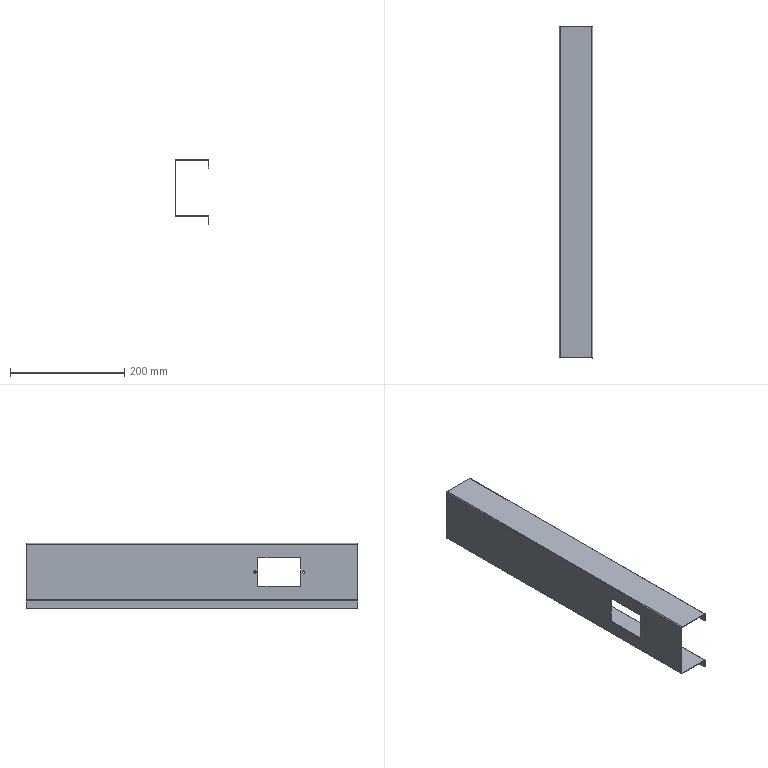Part | SolidWorks | features EdgeFlange 2, FlatPattern 1, ICE 1, SMBaseFlange 1, SheetMetal 1 | 1 solid | 46 faces | box 58.8 x 580 x 113.8 mm | volume 163204 mm3 | plane 34 | cylinder 12 | commonest cylinder face diameters 0.9 x4 3.3 x4 4 x4
STEP:
#1=CARTESIAN_POINT('',(0.,-110.,2.));
#2=VERTEX_POINT('',#1);
#3=CARTESIAN_POINT('',(0.,-110.,-2.));
#4=VERTEX_POINT('',#3);
#5=CARTESIAN_POINT('',(0.,-110.,0.));
#6=DIRECTION('',(1.,0.,0.));
#7=DIRECTION('',(0.,0.,-1.));
#8=AXIS2_PLACEMENT_3D('',#5,#6,#7);
#9=CIRCLE('',#8,2.);
#10=EDGE_CURVE('',#2,#4,#9,.T.);
#11=ORIENTED_EDGE('',*,*,#10,.F.);
#12=CARTESIAN_POINT('',(1.2,-110.,2.));
#13=VERTEX_POINT('',#12);
#14=CARTESIAN_POINT('',(-8.8,-110.,2.));
#15=DIRECTION('',(1.,0.,0.));
#16=VECTOR('',#15,1000.);
#17=LINE('',#14,#16);
#18=EDGE_CURVE('',#2,#13,#17,.T.);
#19=ORIENTED_EDGE('',*,*,#18,.T.);
#20=CARTESIAN_POINT('',(1.2,-110.,-2.));
#21=VERTEX_POINT('',#20);
#22=CARTESIAN_POINT('',(1.2,-110.,0.));
#23=DIRECTION('',(1.,0.,0.));
#24=DIRECTION('',(0.,0.,1.));
#25=AXIS2_PLACEMENT_3D('',#22,#23,#24);
#26=CIRCLE('',#25,2.);
#27=EDGE_CURVE('',#13,#21,#26,.T.);
#28=ORIENTED_EDGE('',*,*,#27,.T.);
#29=CARTESIAN_POINT('',(-8.8,-110.,-2.));
#30=DIRECTION('',(1.,0.,0.));
#31=VECTOR('',#30,1000.);
#32=LINE('',#29,#31);
#33=EDGE_CURVE('',#4,#21,#32,.T.);
#34=ORIENTED_EDGE('',*,*,#33,.F.);
#35=EDGE_LOOP('',(#11,#19,#28,#34));
#36=FACE_OUTER_BOUND('',#35,.T.);
#37=CARTESIAN_POINT('',(-8.8,-110.,0.));
#38=DIRECTION('',(1.,0.,0.));
#39=DIRECTION('',(0.,0.,-1.));
#40=AXIS2_PLACEMENT_3D('',#37,#38,#39);
#41=CYLINDRICAL_SURFACE('',#40,2.);
#42=ADVANCED_FACE('',(#36),#41,.F.);
#43=CARTESIAN_POINT('',(0.,-195.,2.));
#44=VERTEX_POINT('',#43);
#45=CARTESIAN_POINT('',(0.,-195.,-2.));
#46=VERTEX_POINT('',#45);
#47=CARTESIAN_POINT('',(0.,-195.,0.));
#48=DIRECTION('',(1.,0.,0.));
#49=DIRECTION('',(0.,0.,-1.));
#50=AXIS2_PLACEMENT_3D('',#47,#48,#49);
#51=CIRCLE('',#50,2.);
#52=EDGE_CURVE('',#44,#46,#51,.T.);
#53=ORIENTED_EDGE('',*,*,#52,.F.);
#54=CARTESIAN_POINT('',(1.2,-195.,2.));
#55=VERTEX_POINT('',#54);
#56=CARTESIAN_POINT('',(-8.8,-195.,2.));
#57=DIRECTION('',(1.,0.,0.));
#58=VECTOR('',#57,1000.);
#59=LINE('',#56,#58);
#60=EDGE_CURVE('',#44,#55,#59,.T.);
#61=ORIENTED_EDGE('',*,*,#60,.T.);
#62=CARTESIAN_POINT('',(1.2,-195.,-2.));
#63=VERTEX_POINT('',#62);
#64=CARTESIAN_POINT('',(1.2,-195.,0.));
#65=DIRECTION('',(1.,0.,0.));
#66=DIRECTION('',(0.,0.,-1.));
#67=AXIS2_PLACEMENT_3D('',#64,#65,#66);
#68=CIRCLE('',#67,2.);
#69=EDGE_CURVE('',#55,#63,#68,.T.);
#70=ORIENTED_EDGE('',*,*,#69,.T.);
#71=CARTESIAN_POINT('',(-8.8,-195.,-2.));
#72=DIRECTION('',(1.,0.,0.));
#73=VECTOR('',#72,1000.);
#74=LINE('',#71,#73);
#75=EDGE_CURVE('',#46,#63,#74,.T.);
#76=ORIENTED_EDGE('',*,*,#75,.F.);
#77=EDGE_LOOP('',(#53,#61,#70,#76));
#78=FACE_OUTER_BOUND('',#77,.T.);
#79=CARTESIAN_POINT('',(-8.8,-195.,0.));
#80=DIRECTION('',(1.,0.,0.));
#81=DIRECTION('',(0.,0.,-1.));
#82=AXIS2_PLACEMENT_3D('',#79,#80,#81);
#83=CYLINDRICAL_SURFACE('',#82,2.);
#84=ADVANCED_FACE('',(#78),#83,.F.);
#85=CARTESIAN_POINT('',(57.15,290.,-50.));
#86=VERTEX_POINT('',#85);
#87=CARTESIAN_POINT('',(57.15,290.,-48.8));
#88=VERTEX_POINT('',#87);
#89=CARTESIAN_POINT('',(57.15,290.,-50.));
#90=DIRECTION('',(0.,0.,1.));
#91=VECTOR('',#90,1000.);
#92=LINE('',#89,#91);
#93=EDGE_CURVE('',#86,#88,#92,.T.);
#94=ORIENTED_EDGE('',*,*,#93,.F.);
#95=CARTESIAN_POINT('',(1.65,290.,-50.));
#96=VERTEX_POINT('',#95);
#97=CARTESIAN_POINT('',(1.2,290.,-50.));
#98=DIRECTION('',(1.,0.,0.));
#99=VECTOR('',#98,1000.);
#100=LINE('',#97,#99);
#101=EDGE_CURVE('',#96,#86,#100,.T.);
#102=ORIENTED_EDGE('',*,*,#101,.F.);
#103=CARTESIAN_POINT('',(1.65,290.,-48.8));
#104=VERTEX_POINT('',#103);
#105=CARTESIAN_POINT('',(1.65,290.,-48.8));
#106=DIRECTION('',(0.,0.,-1.));
#107=VECTOR('',#106,1000.);
#108=LINE('',#105,#107);
#109=EDGE_CURVE('',#104,#96,#108,.T.);
#110=ORIENTED_EDGE('',*,*,#109,.F.);
#111=CARTESIAN_POINT('',(1.2,290.,-48.8));
#112=DIRECTION('',(1.,0.,0.));
#113=VECTOR('',#112,1000.);
#114=LINE('',#111,#113);
#115=EDGE_CURVE('',#104,#88,#114,.T.);
#116=ORIENTED_EDGE('',*,*,#115,.T.);
#117=EDGE_LOOP('',(#94,#102,#110,#116));
#118=FACE_OUTER_BOUND('',#117,.T.);
#119=CARTESIAN_POINT('',(1.2,290.,-50.));
#120=DIRECTION('',(0.,-1.,0.));
#121=DIRECTION('',(0.,0.,-1.));
#122=AXIS2_PLACEMENT_3D('',#119,#120,#121);
#123=PLANE('',#122);
#124=ADVANCED_FACE('',(#118),#123,.F.);
#125=CARTESIAN_POINT('',(57.15,-290.,-50.));
#126=VERTEX_POINT('',#125);
#127=CARTESIAN_POINT('',(57.15,-290.,-48.8));
#128=VERTEX_POINT('',#127);
#129=CARTESIAN_POINT('',(57.15,-290.,-50.));
#130=DIRECTION('',(0.,0.,1.));
#131=VECTOR('',#130,1000.);
#132=LINE('',#129,#131);
#133=EDGE_CURVE('',#126,#128,#132,.T.);
#134=ORIENTED_EDGE('',*,*,#133,.T.);
#135=CARTESIAN_POINT('',(1.65,-290.,-48.8));
#136=VERTEX_POINT('',#135);
#137=CARTESIAN_POINT('',(58.8,-290.,-48.8));
#138=DIRECTION('',(-1.,0.,0.));
#139=VECTOR('',#138,1000.);
#140=LINE('',#137,#139);
#141=EDGE_CURVE('',#128,#136,#140,.T.);
#142=ORIENTED_EDGE('',*,*,#141,.T.);
#143=CARTESIAN_POINT('',(1.65,-290.,-50.));
#144=VERTEX_POINT('',#143);
#145=CARTESIAN_POINT('',(1.65,-290.,-50.));
#146=DIRECTION('',(0.,0.,-1.));
#147=VECTOR('',#146,1000.);
#148=LINE('',#145,#147);
#149=EDGE_CURVE('',#136,#144,#148,.T.);
#150=ORIENTED_EDGE('',*,*,#149,.T.);
#151=CARTESIAN_POINT('',(1.2,-290.,-50.));
#152=DIRECTION('',(-1.,0.,0.));
#153=VECTOR('',#152,1000.);
#154=LINE('',#151,#153);
#155=EDGE_CURVE('',#126,#144,#154,.T.);
#156=ORIENTED_EDGE('',*,*,#155,.F.);
#157=EDGE_LOOP('',(#134,#142,#150,#156));
#158=FACE_OUTER_BOUND('',#157,.T.);
#159=CARTESIAN_POINT('',(58.8,-290.,-50.));
#160=DIRECTION('',(0.,1.,0.));
#161=DIRECTION('',(0.,0.,1.));
#162=AXIS2_PLACEMENT_3D('',#159,#160,#161);
#163=PLANE('',#162);
#164=ADVANCED_FACE('',(#158),#163,.F.);
#165=ORIENTED_EDGE('',*,*,#101,.T.);
#166=CARTESIAN_POINT('',(57.15,-290.,-50.));
#167=DIRECTION('',(0.,1.,0.));
#168=VECTOR('',#167,1000.);
#169=LINE('',#166,#168);
#170=EDGE_CURVE('',#126,#86,#169,.T.);
#171=ORIENTED_EDGE('',*,*,#170,.F.);
#172=ORIENTED_EDGE('',*,*,#155,.T.);
#173=CARTESIAN_POINT('',(1.65,290.,-50.));
#174=DIRECTION('',(0.,1.,0.));
#175=VECTOR('',#174,1000.);
#176=LINE('',#173,#175);
#177=EDGE_CURVE('',#144,#96,#176,.T.);
#178=ORIENTED_EDGE('',*,*,#177,.T.);
#179=EDGE_LOOP('',(#165,#171,#172,#178));
#180=FACE_OUTER_BOUND('',#179,.T.);
#181=CARTESIAN_POINT('',(1.2,290.,-50.));
#182=DIRECTION('',(0.,0.,-1.));
#183=DIRECTION('',(-1.,0.,0.));
#184=AXIS2_PLACEMENT_3D('',#181,#182,#183);
#185=PLANE('',#184);
#186=ADVANCED_FACE('',(#180),#185,.T.);
#187=CARTESIAN_POINT('',(57.15,-290.,-48.8));
#188=DIRECTION('',(0.,1.,0.));
#189=VECTOR('',#188,1000.);
#190=LINE('',#187,#189);
#191=EDGE_CURVE('',#128,#88,#190,.T.);
#192=ORIENTED_EDGE('',*,*,#191,.T.);
#193=ORIENTED_EDGE('',*,*,#115,.F.);
#194=CARTESIAN_POINT('',(1.65,-290.,-48.8));
#195=DIRECTION('',(0.,1.,0.));
#196=VECTOR('',#195,1000.);
#197=LINE('',#194,#196);
#198=EDGE_CURVE('',#136,#104,#197,.T.);
#199=ORIENTED_EDGE('',*,*,#198,.F.);
#200=ORIENTED_EDGE('',*,*,#141,.F.);
#201=EDGE_LOOP('',(#192,#193,#199,#200));
#202=FACE_OUTER_BOUND('',#201,.T.);
#203=CARTESIAN_POINT('',(1.2,290.,-48.8));
#204=DIRECTION('',(0.,0.,-1.));
#205=DIRECTION('',(-1.,0.,0.));
#206=AXIS2_PLACEMENT_3D('',#203,#204,#205);
#207=PLANE('',#206);
#208=ADVANCED_FACE('',(#202),#207,.F.);
#209=CARTESIAN_POINT('',(57.15,-290.,48.8));
#210=VERTEX_POINT('',#209);
#211=CARTESIAN_POINT('',(57.15,-290.,50.));
#212=VERTEX_POINT('',#211);
#213=CARTESIAN_POINT('',(57.15,-290.,48.8));
#214=DIRECTION('',(0.,0.,1.));
#215=VECTOR('',#214,1000.);
#216=LINE('',#213,#215);
#217=EDGE_CURVE('',#210,#212,#216,.T.);
#218=ORIENTED_EDGE('',*,*,#217,.T.);
#219=CARTESIAN_POINT('',(1.65,-290.,50.));
#220=VERTEX_POINT('',#219);
#221=CARTESIAN_POINT('',(1.2,-290.,50.));
#222=DIRECTION('',(1.,0.,0.));
#223=VECTOR('',#222,1000.);
#224=LINE('',#221,#223);
#225=EDGE_CURVE('',#220,#212,#224,.T.);
#226=ORIENTED_EDGE('',*,*,#225,.F.);
#227=CARTESIAN_POINT('',(1.65,-290.,48.8));
#228=VERTEX_POINT('',#227);
#229=CARTESIAN_POINT('',(1.65,-290.,48.8));
#230=DIRECTION('',(0.,0.,1.));
#231=VECTOR('',#230,1000.);
#232=LINE('',#229,#231);
#233=EDGE_CURVE('',#228,#220,#232,.T.);
#234=ORIENTED_EDGE('',*,*,#233,.F.);
#235=CARTESIAN_POINT('',(58.8,-290.,48.8));
#236=DIRECTION('',(1.,0.,0.));
#237=VECTOR('',#236,1000.);
#238=LINE('',#235,#237);
#239=EDGE_CURVE('',#228,#210,#238,.T.);
#240=ORIENTED_EDGE('',*,*,#239,.T.);
#241=EDGE_LOOP('',(#218,#226,#234,#240));
#242=FACE_OUTER_BOUND('',#241,.T.);
#243=CARTESIAN_POINT('',(58.8,-290.,50.));
#244=DIRECTION('',(0.,1.,0.));
#245=DIRECTION('',(0.,0.,1.));
#246=AXIS2_PLACEMENT_3D('',#243,#244,#245);
#247=PLANE('',#246);
#248=ADVANCED_FACE('',(#242),#247,.F.);
#249=CARTESIAN_POINT('',(57.15,290.,48.8));
#250=VERTEX_POINT('',#249);
#251=CARTESIAN_POINT('',(57.15,290.,50.));
#252=VERTEX_POINT('',#251);
#253=CARTESIAN_POINT('',(57.15,290.,48.8));
#254=DIRECTION('',(0.,0.,1.));
#255=VECTOR('',#254,1000.);
#256=LINE('',#253,#255);
#257=EDGE_CURVE('',#250,#252,#256,.T.);
#258=ORIENTED_EDGE('',*,*,#257,.F.);
#259=CARTESIAN_POINT('',(1.65,290.,48.8));
#260=VERTEX_POINT('',#259);
#261=CARTESIAN_POINT('',(1.2,290.,48.8));
#262=DIRECTION('',(-1.,0.,0.));
#263=VECTOR('',#262,1000.);
#264=LINE('',#261,#263);
#265=EDGE_CURVE('',#250,#260,#264,.T.);
#266=ORIENTED_EDGE('',*,*,#265,.T.);
#267=CARTESIAN_POINT('',(1.65,290.,50.));
#268=VERTEX_POINT('',#267);
#269=CARTESIAN_POINT('',(1.65,290.,50.));
#270=DIRECTION('',(0.,0.,1.));
#271=VECTOR('',#270,1000.);
#272=LINE('',#269,#271);
#273=EDGE_CURVE('',#260,#268,#272,.T.);
#274=ORIENTED_EDGE('',*,*,#273,.T.);
#275=CARTESIAN_POINT('',(1.2,290.,50.));
#276=DIRECTION('',(-1.,0.,0.));
#277=VECTOR('',#276,1000.);
#278=LINE('',#275,#277);
#279=EDGE_CURVE('',#252,#268,#278,.T.);
#280=ORIENTED_EDGE('',*,*,#279,.F.);
#281=EDGE_LOOP('',(#258,#266,#274,#280));
#282=FACE_OUTER_BOUND('',#281,.T.);
#283=CARTESIAN_POINT('',(1.2,290.,50.));
#284=DIRECTION('',(0.,-1.,0.));
#285=DIRECTION('',(0.,0.,-1.));
#286=AXIS2_PLACEMENT_3D('',#283,#284,#285);
#287=PLANE('',#286);
#288=ADVANCED_FACE('',(#282),#287,.F.);
#289=CARTESIAN_POINT('',(57.15,-290.,50.));
#290=DIRECTION('',(0.,1.,0.));
#291=VECTOR('',#290,1000.);
#292=LINE('',#289,#291);
#293=EDGE_CURVE('',#212,#252,#292,.T.);
#294=ORIENTED_EDGE('',*,*,#293,.T.);
#295=ORIENTED_EDGE('',*,*,#279,.T.);
#296=CARTESIAN_POINT('',(1.65,290.,50.));
#297=DIRECTION('',(0.,1.,0.));
#298=VECTOR('',#297,1000.);
#299=LINE('',#296,#298);
#300=EDGE_CURVE('',#220,#268,#299,.T.);
#301=ORIENTED_EDGE('',*,*,#300,.F.);
#302=ORIENTED_EDGE('',*,*,#225,.T.);
#303=EDGE_LOOP('',(#294,#295,#301,#302));
#304=FACE_OUTER_BOUND('',#303,.T.);
#305=CARTESIAN_POINT('',(1.2,-290.,50.));
#306=DIRECTION('',(0.,0.,-1.));
#307=DIRECTION('',(-1.,0.,0.));
#308=AXIS2_PLACEMENT_3D('',#305,#306,#307);
#309=PLANE('',#308);
#310=ADVANCED_FACE('',(#304),#309,.F.);
#311=ORIENTED_EDGE('',*,*,#265,.F.);
#312=CARTESIAN_POINT('',(57.15,-290.,48.8));
#313=DIRECTION('',(0.,1.,0.));
#314=VECTOR('',#313,1000.);
#315=LINE('',#312,#314);
#316=EDGE_CURVE('',#210,#250,#315,.T.);
#317=ORIENTED_EDGE('',*,*,#316,.F.);
#318=ORIENTED_EDGE('',*,*,#239,.F.);
#319=CARTESIAN_POINT('',(1.65,290.,48.8));
#320=DIRECTION('',(0.,-1.,0.));
#321=VECTOR('',#320,1000.);
#322=LINE('',#319,#321);
#323=EDGE_CURVE('',#260,#228,#322,.T.);
#324=ORIENTED_EDGE('',*,*,#323,.F.);
#325=EDGE_LOOP('',(#311,#317,#318,#324));
#326=FACE_OUTER_BOUND('',#325,.T.);
#327=CARTESIAN_POINT('',(1.2,-290.,48.8));
#328=DIRECTION('',(0.,0.,-1.));
#329=DIRECTION('',(-1.,0.,0.));
#330=AXIS2_PLACEMENT_3D('',#327,#328,#329);
#331=PLANE('',#330);
#332=ADVANCED_FACE('',(#326),#331,.T.);
#333=CARTESIAN_POINT('',(1.2,-290.,-48.35));
#334=VERTEX_POINT('',#333);
#335=CARTESIAN_POINT('',(0.,-290.,-48.35));
#336=VERTEX_POINT('',#335);
#337=CARTESIAN_POINT('',(1.2,-290.,-48.35));
#338=DIRECTION('',(-1.,0.,0.));
#339=VECTOR('',#338,1000.);
#340=LINE('',#337,#339);
#341=EDGE_CURVE('',#334,#336,#340,.T.);
#342=ORIENTED_EDGE('',*,*,#341,.F.);
#343=CARTESIAN_POINT('',(1.2,-290.,48.35));
#344=VERTEX_POINT('',#343);
#345=CARTESIAN_POINT('',(1.2,-290.,50.));
#346=DIRECTION('',(0.,0.,-1.));
#347=VECTOR('',#346,1000.);
#348=LINE('',#345,#347);
#349=EDGE_CURVE('',#344,#334,#348,.T.);
#350=ORIENTED_EDGE('',*,*,#349,.F.);
#351=CARTESIAN_POINT('',(0.,-290.,48.35));
#352=VERTEX_POINT('',#351);
#353=CARTESIAN_POINT('',(1.2,-290.,48.35));
#354=DIRECTION('',(-1.,0.,0.));
#355=VECTOR('',#354,1000.);
#356=LINE('',#353,#355);
#357=EDGE_CURVE('',#344,#352,#356,.T.);
#358=ORIENTED_EDGE('',*,*,#357,.T.);
#359=CARTESIAN_POINT('',(0.,-290.,50.));
#360=DIRECTION('',(0.,0.,-1.));
#361=VECTOR('',#360,1000.);
#362=LINE('',#359,#361);
#363=EDGE_CURVE('',#352,#336,#362,.T.);
#364=ORIENTED_EDGE('',*,*,#363,.T.);
#365=EDGE_LOOP('',(#342,#350,#358,#364));
#366=FACE_OUTER_BOUND('',#365,.T.);
#367=CARTESIAN_POINT('',(1.2,-290.,50.));
#368=DIRECTION('',(0.,1.,0.));
#369=DIRECTION('',(0.,0.,1.));
#370=AXIS2_PLACEMENT_3D('',#367,#368,#369);
#371=PLANE('',#370);
#372=ADVANCED_FACE('',(#366),#371,.F.);
#373=CARTESIAN_POINT('',(1.2,290.,-48.35));
#374=VERTEX_POINT('',#373);
#375=CARTESIAN_POINT('',(0.,290.,-48.35));
#376=VERTEX_POINT('',#375);
#377=CARTESIAN_POINT('',(1.2,290.,-48.35));
#378=DIRECTION('',(-1.,0.,0.));
#379=VECTOR('',#378,1000.);
#380=LINE('',#377,#379);
#381=EDGE_CURVE('',#374,#376,#380,.T.);
#382=ORIENTED_EDGE('',*,*,#381,.T.);
#383=CARTESIAN_POINT('',(0.,290.,48.35));
#384=VERTEX_POINT('',#383);
#385=CARTESIAN_POINT('',(0.,290.,50.));
#386=DIRECTION('',(0.,0.,1.));
#387=VECTOR('',#386,1000.);
#388=LINE('',#385,#387);
#389=EDGE_CURVE('',#376,#384,#388,.T.);
#390=ORIENTED_EDGE('',*,*,#389,.T.);
#391=CARTESIAN_POINT('',(1.2,290.,48.35));
#392=VERTEX_POINT('',#391);
#393=CARTESIAN_POINT('',(1.2,290.,48.35));
#394=DIRECTION('',(-1.,0.,0.));
#395=VECTOR('',#394,1000.);
#396=LINE('',#393,#395);
#397=EDGE_CURVE('',#392,#384,#396,.T.);
#398=ORIENTED_EDGE('',*,*,#397,.F.);
#399=CARTESIAN_POINT('',(1.2,290.,50.));
#400=DIRECTION('',(0.,0.,1.));
#401=VECTOR('',#400,1000.);
#402=LINE('',#399,#401);
#403=EDGE_CURVE('',#374,#392,#402,.T.);
#404=ORIENTED_EDGE('',*,*,#403,.F.);
#405=EDGE_LOOP('',(#382,#390,#398,#404));
#406=FACE_OUTER_BOUND('',#405,.T.);
#407=CARTESIAN_POINT('',(1.2,290.,50.));
#408=DIRECTION('',(0.,-1.,0.));
#409=DIRECTION('',(0.,0.,-1.));
#410=AXIS2_PLACEMENT_3D('',#407,#408,#409);
#411=PLANE('',#410);
#412=ADVANCED_FACE('',(#406),#411,.F.);
#413=CARTESIAN_POINT('',(1.2,-110.,0.));
#414=DIRECTION('',(1.,0.,0.));
#415=DIRECTION('',(0.,0.,1.));
#416=AXIS2_PLACEMENT_3D('',#413,#414,#415);
#417=CIRCLE('',#416,2.);
#418=EDGE_CURVE('',#21,#13,#417,.T.);
#419=ORIENTED_EDGE('',*,*,#418,.F.);
#420=ORIENTED_EDGE('',*,*,#27,.F.);
#421=EDGE_LOOP('',(#419,#420));
#422=FACE_BOUND('',#421,.T.);
#423=CARTESIAN_POINT('',(1.2,-195.,0.));
#424=DIRECTION('',(1.,0.,0.));
#425=DIRECTION('',(0.,0.,-1.));
#426=AXIS2_PLACEMENT_3D('',#423,#424,#425);
#427=CIRCLE('',#426,2.);
#428=EDGE_CURVE('',#63,#55,#427,.T.);
#429=ORIENTED_EDGE('',*,*,#428,.F.);
#430=ORIENTED_EDGE('',*,*,#69,.F.);
#431=EDGE_LOOP('',(#429,#430));
#432=FACE_BOUND('',#431,.T.);
#433=CARTESIAN_POINT('',(1.2,-115.,25.));
#434=VERTEX_POINT('',#433);
#435=CARTESIAN_POINT('',(1.2,-190.,25.));
#436=VERTEX_POINT('',#435);
#437=CARTESIAN_POINT('',(1.2,-115.,25.));
#438=DIRECTION('',(0.,-1.,0.));
#439=VECTOR('',#438,1000.);
#440=LINE('',#437,#439);
#441=EDGE_CURVE('',#434,#436,#440,.T.);
#442=ORIENTED_EDGE('',*,*,#441,.F.);
#443=CARTESIAN_POINT('',(1.2,-115.,-25.));
#444=VERTEX_POINT('',#443);
#445=CARTESIAN_POINT('',(1.2,-115.,25.));
#446=DIRECTION('',(0.,0.,1.));
#447=VECTOR('',#446,1000.);
#448=LINE('',#445,#447);
#449=EDGE_CURVE('',#444,#434,#448,.T.);
#450=ORIENTED_EDGE('',*,*,#449,.F.);
#451=CARTESIAN_POINT('',(1.2,-190.,-25.));
#452=VERTEX_POINT('',#451);
#453=CARTESIAN_POINT('',(1.2,-115.,-25.));
#454=DIRECTION('',(0.,1.,0.));
#455=VECTOR('',#454,1000.);
#456=LINE('',#453,#455);
#457=EDGE_CURVE('',#452,#444,#456,.T.);
#458=ORIENTED_EDGE('',*,*,#457,.F.);
#459=CARTESIAN_POINT('',(1.2,-190.,25.));
#460=DIRECTION('',(0.,0.,-1.));
#461=VECTOR('',#460,1000.);
#462=LINE('',#459,#461);
#463=EDGE_CURVE('',#436,#452,#462,.T.);
#464=ORIENTED_EDGE('',*,*,#463,.F.);
#465=EDGE_LOOP('',(#442,#450,#458,#464));
#466=FACE_BOUND('',#465,.T.);
#467=ORIENTED_EDGE('',*,*,#349,.T.);
#468=CARTESIAN_POINT('',(1.2,290.,-48.35));
#469=DIRECTION('',(0.,-1.,0.));
#470=VECTOR('',#469,1000.);
#471=LINE('',#468,#470);
#472=EDGE_CURVE('',#374,#334,#471,.T.);
#473=ORIENTED_EDGE('',*,*,#472,.F.);
#474=ORIENTED_EDGE('',*,*,#403,.T.);
#475=CARTESIAN_POINT('',(1.2,-290.,48.35));
#476=DIRECTION('',(0.,1.,0.));
#477=VECTOR('',#476,1000.);
#478=LINE('',#475,#477);
#479=EDGE_CURVE('',#344,#392,#478,.T.);
#480=ORIENTED_EDGE('',*,*,#479,.F.);
#481=EDGE_LOOP('',(#467,#473,#474,#480));
#482=FACE_OUTER_BOUND('',#481,.T.);
#483=CARTESIAN_POINT('',(1.2,-290.,50.));
#484=DIRECTION('',(1.,0.,0.));
#485=DIRECTION('',(0.,0.,-1.));
#486=AXIS2_PLACEMENT_3D('',#483,#484,#485);
#487=PLANE('',#486);
#488=ADVANCED_FACE('',(#422,#432,#466,#482),#487,.T.);
#489=CARTESIAN_POINT('',(0.,-110.,0.));
#490=DIRECTION('',(1.,0.,0.));
#491=DIRECTION('',(0.,0.,-1.));
#492=AXIS2_PLACEMENT_3D('',#489,#490,#491);
#493=CIRCLE('',#492,2.);
#494=EDGE_CURVE('',#4,#2,#493,.T.);
#495=ORIENTED_EDGE('',*,*,#494,.T.);
#496=ORIENTED_EDGE('',*,*,#10,.T.);
#497=EDGE_LOOP('',(#495,#496));
#498=FACE_BOUND('',#497,.T.);
#499=CARTESIAN_POINT('',(0.,-195.,0.));
#500=DIRECTION('',(1.,0.,0.));
#501=DIRECTION('',(0.,0.,-1.));
#502=AXIS2_PLACEMENT_3D('',#499,#500,#501);
#503=CIRCLE('',#502,2.);
#504=EDGE_CURVE('',#46,#44,#503,.T.);
#505=ORIENTED_EDGE('',*,*,#504,.T.);
#506=ORIENTED_EDGE('',*,*,#52,.T.);
#507=EDGE_LOOP('',(#505,#506));
#508=FACE_BOUND('',#507,.T.);
#509=CARTESIAN_POINT('',(0.,-115.,-25.));
#510=VERTEX_POINT('',#509);
#511=CARTESIAN_POINT('',(0.,-115.,25.));
#512=VERTEX_POINT('',#511);
#513=CARTESIAN_POINT('',(0.,-115.,50.));
#514=DIRECTION('',(0.,0.,1.));
#515=VECTOR('',#514,1000.);
#516=LINE('',#513,#515);
#517=EDGE_CURVE('',#510,#512,#516,.T.);
#518=ORIENTED_EDGE('',*,*,#517,.T.);
#519=CARTESIAN_POINT('',(0.,-190.,25.));
#520=VERTEX_POINT('',#519);
#521=CARTESIAN_POINT('',(0.,-290.,25.));
#522=DIRECTION('',(0.,-1.,0.));
#523=VECTOR('',#522,1000.);
#524=LINE('',#521,#523);
#525=EDGE_CURVE('',#512,#520,#524,.T.);
#526=ORIENTED_EDGE('',*,*,#525,.T.);
#527=CARTESIAN_POINT('',(0.,-190.,-25.));
#528=VERTEX_POINT('',#527);
#529=CARTESIAN_POINT('',(0.,-190.,50.));
#530=DIRECTION('',(0.,0.,-1.));
#531=VECTOR('',#530,1000.);
#532=LINE('',#529,#531);
#533=EDGE_CURVE('',#520,#528,#532,.T.);
#534=ORIENTED_EDGE('',*,*,#533,.T.);
#535=CARTESIAN_POINT('',(0.,-290.,-25.));
#536=DIRECTION('',(0.,1.,0.));
#537=VECTOR('',#536,1000.);
#538=LINE('',#535,#537);
#539=EDGE_CURVE('',#528,#510,#538,.T.);
#540=ORIENTED_EDGE('',*,*,#539,.T.);
#541=EDGE_LOOP('',(#518,#526,#534,#540));
#542=FACE_BOUND('',#541,.T.);
#543=CARTESIAN_POINT('',(0.,290.,-48.35));
#544=DIRECTION('',(0.,-1.,0.));
#545=VECTOR('',#544,1000.);
#546=LINE('',#543,#545);
#547=EDGE_CURVE('',#376,#336,#546,.T.);
#548=ORIENTED_EDGE('',*,*,#547,.T.);
#549=ORIENTED_EDGE('',*,*,#363,.F.);
#550=CARTESIAN_POINT('',(0.,-290.,48.35));
#551=DIRECTION('',(0.,1.,0.));
#552=VECTOR('',#551,1000.);
#553=LINE('',#550,#552);
#554=EDGE_CURVE('',#352,#384,#553,.T.);
#555=ORIENTED_EDGE('',*,*,#554,.T.);
#556=ORIENTED_EDGE('',*,*,#389,.F.);
#557=EDGE_LOOP('',(#548,#549,#555,#556));
#558=FACE_OUTER_BOUND('',#557,.T.);
#559=CARTESIAN_POINT('',(0.,-290.,50.));
#560=DIRECTION('',(1.,0.,0.));
#561=DIRECTION('',(0.,0.,-1.));
#562=AXIS2_PLACEMENT_3D('',#559,#560,#561);
#563=PLANE('',#562);
#564=ADVANCED_FACE('',(#498,#508,#542,#558),#563,.F.);
#565=ORIENTED_EDGE('',*,*,#273,.F.);
#566=CARTESIAN_POINT('',(1.65,290.,48.35));
#567=DIRECTION('',(0.,1.,0.));
#568=DIRECTION('',(0.,0.,-1.));
#569=AXIS2_PLACEMENT_3D('',#566,#567,#568);
#570=CIRCLE('',#569,0.45);
#571=EDGE_CURVE('',#392,#260,#570,.T.);
#572=ORIENTED_EDGE('',*,*,#571,.F.);
#573=ORIENTED_EDGE('',*,*,#397,.T.);
#574=CARTESIAN_POINT('',(1.65,290.,48.35));
#575=DIRECTION('',(0.,1.,0.));
#576=DIRECTION('',(0.,0.,-1.));
#577=AXIS2_PLACEMENT_3D('',#574,#575,#576);
#578=CIRCLE('',#577,1.65);
#579=EDGE_CURVE('',#384,#268,#578,.T.);
#580=ORIENTED_EDGE('',*,*,#579,.T.);
#581=EDGE_LOOP('',(#565,#572,#573,#580));
#582=FACE_OUTER_BOUND('',#581,.T.);
#583=CARTESIAN_POINT('',(1.65,290.,48.35));
#584=DIRECTION('',(0.,1.,0.));
#585=DIRECTION('',(0.,0.,1.));
#586=AXIS2_PLACEMENT_3D('',#583,#584,#585);
#587=PLANE('',#586);
#588=ADVANCED_FACE('',(#582),#587,.T.);
#589=ORIENTED_EDGE('',*,*,#554,.F.);
#590=CARTESIAN_POINT('',(1.65,-290.,48.35));
#591=DIRECTION('',(0.,-1.,0.));
#592=DIRECTION('',(0.,0.,-1.));
#593=AXIS2_PLACEMENT_3D('',#590,#591,#592);
#594=CIRCLE('',#593,1.65);
#595=EDGE_CURVE('',#220,#352,#594,.T.);
#596=ORIENTED_EDGE('',*,*,#595,.F.);
#597=ORIENTED_EDGE('',*,*,#300,.T.);
#598=ORIENTED_EDGE('',*,*,#579,.F.);
#599=EDGE_LOOP('',(#589,#596,#597,#598));
#600=FACE_OUTER_BOUND('',#599,.T.);
#601=CARTESIAN_POINT('',(1.65,-290.,48.35));
#602=DIRECTION('',(0.,-1.,0.));
#603=DIRECTION('',(0.,0.,1.));
#604=AXIS2_PLACEMENT_3D('',#601,#602,#603);
#605=CYLINDRICAL_SURFACE('',#604,1.65);
#606=ADVANCED_FACE('',(#600),#605,.T.);
#607=CARTESIAN_POINT('',(1.65,-290.,48.35));
#608=DIRECTION('',(0.,-1.,0.));
#609=DIRECTION('',(0.,0.,-1.));
#610=AXIS2_PLACEMENT_3D('',#607,#608,#609);
#611=CIRCLE('',#610,0.45);
#612=EDGE_CURVE('',#228,#344,#611,.T.);
#613=ORIENTED_EDGE('',*,*,#612,.F.);
#614=ORIENTED_EDGE('',*,*,#233,.T.);
#615=ORIENTED_EDGE('',*,*,#595,.T.);
#616=ORIENTED_EDGE('',*,*,#357,.F.);
#617=EDGE_LOOP('',(#613,#614,#615,#616));
#618=FACE_OUTER_BOUND('',#617,.T.);
#619=CARTESIAN_POINT('',(1.65,-290.,48.35));
#620=DIRECTION('',(0.,1.,0.));
#621=DIRECTION('',(0.,0.,1.));
#622=AXIS2_PLACEMENT_3D('',#619,#620,#621);
#623=PLANE('',#622);
#624=ADVANCED_FACE('',(#618),#623,.F.);
#625=ORIENTED_EDGE('',*,*,#479,.T.);
#626=ORIENTED_EDGE('',*,*,#571,.T.);
#627=ORIENTED_EDGE('',*,*,#323,.T.);
#628=ORIENTED_EDGE('',*,*,#612,.T.);
#629=EDGE_LOOP('',(#625,#626,#627,#628));
#630=FACE_OUTER_BOUND('',#629,.T.);
#631=CARTESIAN_POINT('',(1.65,-290.,48.35));
#632=DIRECTION('',(0.,-1.,0.));
#633=DIRECTION('',(0.,0.,1.));
#634=AXIS2_PLACEMENT_3D('',#631,#632,#633);
#635=CYLINDRICAL_SURFACE('',#634,0.45);
#636=ADVANCED_FACE('',(#630),#635,.F.);
#637=ORIENTED_EDGE('',*,*,#149,.F.);
#638=CARTESIAN_POINT('',(1.65,-290.,-48.35));
#639=DIRECTION('',(0.,-1.,0.));
#640=DIRECTION('',(0.,0.,1.));
#641=AXIS2_PLACEMENT_3D('',#638,#639,#640);
#642=CIRCLE('',#641,0.45);
#643=EDGE_CURVE('',#334,#136,#642,.T.);
#644=ORIENTED_EDGE('',*,*,#643,.F.);
#645=ORIENTED_EDGE('',*,*,#341,.T.);
#646=CARTESIAN_POINT('',(1.65,-290.,-48.35));
#647=DIRECTION('',(0.,-1.,0.));
#648=DIRECTION('',(0.,0.,1.));
#649=AXIS2_PLACEMENT_3D('',#646,#647,#648);
#650=CIRCLE('',#649,1.65);
#651=EDGE_CURVE('',#336,#144,#650,.T.);
#652=ORIENTED_EDGE('',*,*,#651,.T.);
#653=EDGE_LOOP('',(#637,#644,#645,#652));
#654=FACE_OUTER_BOUND('',#653,.T.);
#655=CARTESIAN_POINT('',(1.65,-290.,-48.35));
#656=DIRECTION('',(0.,-1.,0.));
#657=DIRECTION('',(0.,0.,-1.));
#658=AXIS2_PLACEMENT_3D('',#655,#656,#657);
#659=PLANE('',#658);
#660=ADVANCED_FACE('',(#654),#659,.T.);
#661=ORIENTED_EDGE('',*,*,#547,.F.);
#662=CARTESIAN_POINT('',(1.65,290.,-48.35));
#663=DIRECTION('',(0.,1.,0.));
#664=DIRECTION('',(0.,0.,1.));
#665=AXIS2_PLACEMENT_3D('',#662,#663,#664);
#666=CIRCLE('',#665,1.65);
#667=EDGE_CURVE('',#96,#376,#666,.T.);
#668=ORIENTED_EDGE('',*,*,#667,.F.);
#669=ORIENTED_EDGE('',*,*,#177,.F.);
#670=ORIENTED_EDGE('',*,*,#651,.F.);
#671=EDGE_LOOP('',(#661,#668,#669,#670));
#672=FACE_OUTER_BOUND('',#671,.T.);
#673=CARTESIAN_POINT('',(1.65,290.,-48.35));
#674=DIRECTION('',(0.,1.,0.));
#675=DIRECTION('',(0.,0.,-1.));
#676=AXIS2_PLACEMENT_3D('',#673,#674,#675);
#677=CYLINDRICAL_SURFACE('',#676,1.65);
#678=ADVANCED_FACE('',(#672),#677,.T.);
#679=CARTESIAN_POINT('',(1.65,290.,-48.35));
#680=DIRECTION('',(0.,1.,0.));
#681=DIRECTION('',(0.,0.,1.));
#682=AXIS2_PLACEMENT_3D('',#679,#680,#681);
#683=CIRCLE('',#682,0.45);
#684=EDGE_CURVE('',#104,#374,#683,.T.);
#685=ORIENTED_EDGE('',*,*,#684,.F.);
#686=ORIENTED_EDGE('',*,*,#109,.T.);
#687=ORIENTED_EDGE('',*,*,#667,.T.);
#688=ORIENTED_EDGE('',*,*,#381,.F.);
#689=EDGE_LOOP('',(#685,#686,#687,#688));
#690=FACE_OUTER_BOUND('',#689,.T.);
#691=CARTESIAN_POINT('',(1.65,290.,-48.35));
#692=DIRECTION('',(0.,-1.,0.));
#693=DIRECTION('',(0.,0.,-1.));
#694=AXIS2_PLACEMENT_3D('',#691,#692,#693);
#695=PLANE('',#694);
#696=ADVANCED_FACE('',(#690),#695,.F.);
#697=ORIENTED_EDGE('',*,*,#472,.T.);
#698=ORIENTED_EDGE('',*,*,#643,.T.);
#699=ORIENTED_EDGE('',*,*,#198,.T.);
#700=ORIENTED_EDGE('',*,*,#684,.T.);
#701=EDGE_LOOP('',(#697,#698,#699,#700));
#702=FACE_OUTER_BOUND('',#701,.T.);
#703=CARTESIAN_POINT('',(1.65,290.,-48.35));
#704=DIRECTION('',(0.,1.,0.));
#705=DIRECTION('',(0.,0.,-1.));
#706=AXIS2_PLACEMENT_3D('',#703,#704,#705);
#707=CYLINDRICAL_SURFACE('',#706,0.45);
#708=ADVANCED_FACE('',(#702),#707,.F.);
#709=CARTESIAN_POINT('',(57.6,290.,48.35));
#710=VERTEX_POINT('',#709);
#711=CARTESIAN_POINT('',(58.8,290.,48.35));
#712=VERTEX_POINT('',#711);
#713=CARTESIAN_POINT('',(58.8,290.,48.35));
#714=DIRECTION('',(1.,0.,0.));
#715=VECTOR('',#714,1000.);
#716=LINE('',#713,#715);
#717=EDGE_CURVE('',#710,#712,#716,.T.);
#718=ORIENTED_EDGE('',*,*,#717,.F.);
#719=CARTESIAN_POINT('',(57.15,290.,48.35));
#720=DIRECTION('',(0.,1.,0.));
#721=DIRECTION('',(0.,0.,-1.));
#722=AXIS2_PLACEMENT_3D('',#719,#720,#721);
#723=CIRCLE('',#722,0.45);
#724=EDGE_CURVE('',#250,#710,#723,.T.);
#725=ORIENTED_EDGE('',*,*,#724,.F.);
#726=ORIENTED_EDGE('',*,*,#257,.T.);
#727=CARTESIAN_POINT('',(57.15,290.,48.35));
#728=DIRECTION('',(0.,1.,0.));
#729=DIRECTION('',(0.,0.,-1.));
#730=AXIS2_PLACEMENT_3D('',#727,#728,#729);
#731=CIRCLE('',#730,1.65);
#732=EDGE_CURVE('',#252,#712,#731,.T.);
#733=ORIENTED_EDGE('',*,*,#732,.T.);
#734=EDGE_LOOP('',(#718,#725,#726,#733));
#735=FACE_OUTER_BOUND('',#734,.T.);
#736=CARTESIAN_POINT('',(57.15,290.,48.35));
#737=DIRECTION('',(0.,1.,0.));
#738=DIRECTION('',(0.,0.,1.));
#739=AXIS2_PLACEMENT_3D('',#736,#737,#738);
#740=PLANE('',#739);
#741=ADVANCED_FACE('',(#735),#740,.T.);
#742=ORIENTED_EDGE('',*,*,#293,.F.);
#743=CARTESIAN_POINT('',(58.8,-290.,48.35));
#744=VERTEX_POINT('',#743);
#745=CARTESIAN_POINT('',(57.15,-290.,48.35));
#746=DIRECTION('',(0.,-1.,0.));
#747=DIRECTION('',(0.,0.,-1.));
#748=AXIS2_PLACEMENT_3D('',#745,#746,#747);
#749=CIRCLE('',#748,1.65);
#750=EDGE_CURVE('',#744,#212,#749,.T.);
#751=ORIENTED_EDGE('',*,*,#750,.F.);
#752=CARTESIAN_POINT('',(58.8,290.,48.35));
#753=DIRECTION('',(0.,1.,0.));
#754=VECTOR('',#753,1000.);
#755=LINE('',#752,#754);
#756=EDGE_CURVE('',#744,#712,#755,.T.);
#757=ORIENTED_EDGE('',*,*,#756,.T.);
#758=ORIENTED_EDGE('',*,*,#732,.F.);
#759=EDGE_LOOP('',(#742,#751,#757,#758));
#760=FACE_OUTER_BOUND('',#759,.T.);
#761=CARTESIAN_POINT('',(57.15,-290.,48.35));
#762=DIRECTION('',(0.,-1.,0.));
#763=DIRECTION('',(1.,0.,0.));
#764=AXIS2_PLACEMENT_3D('',#761,#762,#763);
#765=CYLINDRICAL_SURFACE('',#764,1.65);
#766=ADVANCED_FACE('',(#760),#765,.T.);
#767=CARTESIAN_POINT('',(57.6,-290.,48.35));
#768=VERTEX_POINT('',#767);
#769=CARTESIAN_POINT('',(57.15,-290.,48.35));
#770=DIRECTION('',(0.,-1.,0.));
#771=DIRECTION('',(0.,0.,-1.));
#772=AXIS2_PLACEMENT_3D('',#769,#770,#771);
#773=CIRCLE('',#772,0.45);
#774=EDGE_CURVE('',#768,#210,#773,.T.);
#775=ORIENTED_EDGE('',*,*,#774,.F.);
#776=CARTESIAN_POINT('',(57.6,-290.,48.35));
#777=DIRECTION('',(1.,0.,0.));
#778=VECTOR('',#777,1000.);
#779=LINE('',#776,#778);
#780=EDGE_CURVE('',#768,#744,#779,.T.);
#781=ORIENTED_EDGE('',*,*,#780,.T.);
#782=ORIENTED_EDGE('',*,*,#750,.T.);
#783=ORIENTED_EDGE('',*,*,#217,.F.);
#784=EDGE_LOOP('',(#775,#781,#782,#783));
#785=FACE_OUTER_BOUND('',#784,.T.);
#786=CARTESIAN_POINT('',(57.15,-290.,48.35));
#787=DIRECTION('',(0.,1.,0.));
#788=DIRECTION('',(0.,0.,1.));
#789=AXIS2_PLACEMENT_3D('',#786,#787,#788);
#790=PLANE('',#789);
#791=ADVANCED_FACE('',(#785),#790,.F.);
#792=ORIENTED_EDGE('',*,*,#316,.T.);
#793=ORIENTED_EDGE('',*,*,#724,.T.);
#794=CARTESIAN_POINT('',(57.6,290.,48.35));
#795=DIRECTION('',(0.,-1.,0.));
#796=VECTOR('',#795,1000.);
#797=LINE('',#794,#796);
#798=EDGE_CURVE('',#710,#768,#797,.T.);
#799=ORIENTED_EDGE('',*,*,#798,.T.);
#800=ORIENTED_EDGE('',*,*,#774,.T.);
#801=EDGE_LOOP('',(#792,#793,#799,#800));
#802=FACE_OUTER_BOUND('',#801,.T.);
#803=CARTESIAN_POINT('',(57.15,-290.,48.35));
#804=DIRECTION('',(0.,-1.,0.));
#805=DIRECTION('',(1.,0.,0.));
#806=AXIS2_PLACEMENT_3D('',#803,#804,#805);
#807=CYLINDRICAL_SURFACE('',#806,0.45);
#808=ADVANCED_FACE('',(#802),#807,.F.);
#809=CARTESIAN_POINT('',(58.8,-290.,35.));
#810=VERTEX_POINT('',#809);
#811=CARTESIAN_POINT('',(58.8,-290.,35.));
#812=DIRECTION('',(0.,0.,1.));
#813=VECTOR('',#812,1000.);
#814=LINE('',#811,#813);
#815=EDGE_CURVE('',#810,#744,#814,.T.);
#816=ORIENTED_EDGE('',*,*,#815,.T.);
#817=ORIENTED_EDGE('',*,*,#780,.F.);
#818=CARTESIAN_POINT('',(57.6,-290.,35.));
#819=VERTEX_POINT('',#818);
#820=CARTESIAN_POINT('',(57.6,-290.,48.8));
#821=DIRECTION('',(0.,0.,1.));
#822=VECTOR('',#821,1000.);
#823=LINE('',#820,#822);
#824=EDGE_CURVE('',#819,#768,#823,.T.);
#825=ORIENTED_EDGE('',*,*,#824,.F.);
#826=CARTESIAN_POINT('',(58.8,-290.,35.));
#827=DIRECTION('',(-1.,0.,0.));
#828=VECTOR('',#827,1000.);
#829=LINE('',#826,#828);
#830=EDGE_CURVE('',#810,#819,#829,.T.);
#831=ORIENTED_EDGE('',*,*,#830,.F.);
#832=EDGE_LOOP('',(#816,#817,#825,#831));
#833=FACE_OUTER_BOUND('',#832,.T.);
#834=CARTESIAN_POINT('',(58.8,-290.,35.));
#835=DIRECTION('',(0.,-1.,0.));
#836=DIRECTION('',(1.,0.,0.));
#837=AXIS2_PLACEMENT_3D('',#834,#835,#836);
#838=PLANE('',#837);
#839=ADVANCED_FACE('',(#833),#838,.T.);
#840=CARTESIAN_POINT('',(57.6,290.,35.));
#841=VERTEX_POINT('',#840);
#842=CARTESIAN_POINT('',(57.6,290.,48.8));
#843=DIRECTION('',(0.,0.,-1.));
#844=VECTOR('',#843,1000.);
#845=LINE('',#842,#844);
#846=EDGE_CURVE('',#710,#841,#845,.T.);
#847=ORIENTED_EDGE('',*,*,#846,.F.);
#848=ORIENTED_EDGE('',*,*,#717,.T.);
#849=CARTESIAN_POINT('',(58.8,290.,35.));
#850=VERTEX_POINT('',#849);
#851=CARTESIAN_POINT('',(58.8,290.,48.8));
#852=DIRECTION('',(0.,0.,-1.));
#853=VECTOR('',#852,1000.);
#854=LINE('',#851,#853);
#855=EDGE_CURVE('',#712,#850,#854,.T.);
#856=ORIENTED_EDGE('',*,*,#855,.T.);
#857=CARTESIAN_POINT('',(58.8,290.,35.));
#858=DIRECTION('',(-1.,0.,0.));
#859=VECTOR('',#858,1000.);
#860=LINE('',#857,#859);
#861=EDGE_CURVE('',#850,#841,#860,.T.);
#862=ORIENTED_EDGE('',*,*,#861,.T.);
#863=EDGE_LOOP('',(#847,#848,#856,#862));
#864=FACE_OUTER_BOUND('',#863,.T.);
#865=CARTESIAN_POINT('',(58.8,290.,48.8));
#866=DIRECTION('',(0.,1.,0.));
#867=DIRECTION('',(-1.,0.,0.));
#868=AXIS2_PLACEMENT_3D('',#865,#866,#867);
#869=PLANE('',#868);
#870=ADVANCED_FACE('',(#864),#869,.T.);
#871=ORIENTED_EDGE('',*,*,#756,.F.);
#872=ORIENTED_EDGE('',*,*,#815,.F.);
#873=CARTESIAN_POINT('',(58.8,290.,35.));
#874=DIRECTION('',(0.,-1.,0.));
#875=VECTOR('',#874,1000.);
#876=LINE('',#873,#875);
#877=EDGE_CURVE('',#850,#810,#876,.T.);
#878=ORIENTED_EDGE('',*,*,#877,.F.);
#879=ORIENTED_EDGE('',*,*,#855,.F.);
#880=EDGE_LOOP('',(#871,#872,#878,#879));
#881=FACE_OUTER_BOUND('',#880,.T.);
#882=CARTESIAN_POINT('',(58.8,290.,48.8));
#883=DIRECTION('',(-1.,0.,0.));
#884=DIRECTION('',(0.,0.,1.));
#885=AXIS2_PLACEMENT_3D('',#882,#883,#884);
#886=PLANE('',#885);
#887=ADVANCED_FACE('',(#881),#886,.F.);
#888=ORIENTED_EDGE('',*,*,#824,.T.);
#889=ORIENTED_EDGE('',*,*,#798,.F.);
#890=ORIENTED_EDGE('',*,*,#846,.T.);
#891=CARTESIAN_POINT('',(57.6,290.,35.));
#892=DIRECTION('',(0.,-1.,0.));
#893=VECTOR('',#892,1000.);
#894=LINE('',#891,#893);
#895=EDGE_CURVE('',#841,#819,#894,.T.);
#896=ORIENTED_EDGE('',*,*,#895,.T.);
#897=EDGE_LOOP('',(#888,#889,#890,#896));
#898=FACE_OUTER_BOUND('',#897,.T.);
#899=CARTESIAN_POINT('',(57.6,290.,48.8));
#900=DIRECTION('',(-1.,0.,0.));
#901=DIRECTION('',(0.,0.,1.));
#902=AXIS2_PLACEMENT_3D('',#899,#900,#901);
#903=PLANE('',#902);
#904=ADVANCED_FACE('',(#898),#903,.T.);
#905=ORIENTED_EDGE('',*,*,#895,.F.);
#906=ORIENTED_EDGE('',*,*,#861,.F.);
#907=ORIENTED_EDGE('',*,*,#877,.T.);
#908=ORIENTED_EDGE('',*,*,#830,.T.);
#909=EDGE_LOOP('',(#905,#906,#907,#908));
#910=FACE_OUTER_BOUND('',#909,.T.);
#911=CARTESIAN_POINT('',(58.8,290.,35.));
#912=DIRECTION('',(0.,0.,-1.));
#913=DIRECTION('',(-1.,0.,0.));
#914=AXIS2_PLACEMENT_3D('',#911,#912,#913);
#915=PLANE('',#914);
#916=ADVANCED_FACE('',(#910),#915,.T.);
#917=CARTESIAN_POINT('',(57.6,290.,-50.45));
#918=VERTEX_POINT('',#917);
#919=CARTESIAN_POINT('',(58.8,290.,-50.45));
#920=VERTEX_POINT('',#919);
#921=CARTESIAN_POINT('',(58.8,290.,-50.45));
#922=DIRECTION('',(1.,0.,0.));
#923=VECTOR('',#922,1000.);
#924=LINE('',#921,#923);
#925=EDGE_CURVE('',#918,#920,#924,.T.);
#926=ORIENTED_EDGE('',*,*,#925,.F.);
#927=CARTESIAN_POINT('',(57.15,290.,-50.45));
#928=DIRECTION('',(0.,1.,0.));
#929=DIRECTION('',(0.,0.,-1.));
#930=AXIS2_PLACEMENT_3D('',#927,#928,#929);
#931=CIRCLE('',#930,0.45);
#932=EDGE_CURVE('',#86,#918,#931,.T.);
#933=ORIENTED_EDGE('',*,*,#932,.F.);
#934=ORIENTED_EDGE('',*,*,#93,.T.);
#935=CARTESIAN_POINT('',(57.15,290.,-50.45));
#936=DIRECTION('',(0.,1.,0.));
#937=DIRECTION('',(0.,0.,-1.));
#938=AXIS2_PLACEMENT_3D('',#935,#936,#937);
#939=CIRCLE('',#938,1.65);
#940=EDGE_CURVE('',#88,#920,#939,.T.);
#941=ORIENTED_EDGE('',*,*,#940,.T.);
#942=EDGE_LOOP('',(#926,#933,#934,#941));
#943=FACE_OUTER_BOUND('',#942,.T.);
#944=CARTESIAN_POINT('',(57.15,290.,-50.45));
#945=DIRECTION('',(0.,1.,0.));
#946=DIRECTION('',(0.,0.,1.));
#947=AXIS2_PLACEMENT_3D('',#944,#945,#946);
#948=PLANE('',#947);
#949=ADVANCED_FACE('',(#943),#948,.T.);
#950=ORIENTED_EDGE('',*,*,#191,.F.);
#951=CARTESIAN_POINT('',(58.8,-290.,-50.45));
#952=VERTEX_POINT('',#951);
#953=CARTESIAN_POINT('',(57.15,-290.,-50.45));
#954=DIRECTION('',(0.,-1.,0.));
#955=DIRECTION('',(0.,0.,-1.));
#956=AXIS2_PLACEMENT_3D('',#953,#954,#955);
#957=CIRCLE('',#956,1.65);
#958=EDGE_CURVE('',#952,#128,#957,.T.);
#959=ORIENTED_EDGE('',*,*,#958,.F.);
#960=CARTESIAN_POINT('',(58.8,290.,-50.45));
#961=DIRECTION('',(0.,1.,0.));
#962=VECTOR('',#961,1000.);
#963=LINE('',#960,#962);
#964=EDGE_CURVE('',#952,#920,#963,.T.);
#965=ORIENTED_EDGE('',*,*,#964,.T.);
#966=ORIENTED_EDGE('',*,*,#940,.F.);
#967=EDGE_LOOP('',(#950,#959,#965,#966));
#968=FACE_OUTER_BOUND('',#967,.T.);
#969=CARTESIAN_POINT('',(57.15,-290.,-50.45));
#970=DIRECTION('',(0.,-1.,0.));
#971=DIRECTION('',(1.,0.,0.));
#972=AXIS2_PLACEMENT_3D('',#969,#970,#971);
#973=CYLINDRICAL_SURFACE('',#972,1.65);
#974=ADVANCED_FACE('',(#968),#973,.T.);
#975=CARTESIAN_POINT('',(57.6,-290.,-50.45));
#976=VERTEX_POINT('',#975);
#977=CARTESIAN_POINT('',(57.15,-290.,-50.45));
#978=DIRECTION('',(0.,-1.,0.));
#979=DIRECTION('',(0.,0.,-1.));
#980=AXIS2_PLACEMENT_3D('',#977,#978,#979);
#981=CIRCLE('',#980,0.45);
#982=EDGE_CURVE('',#976,#126,#981,.T.);
#983=ORIENTED_EDGE('',*,*,#982,.F.);
#984=CARTESIAN_POINT('',(57.6,-290.,-50.45));
#985=DIRECTION('',(1.,0.,0.));
#986=VECTOR('',#985,1000.);
#987=LINE('',#984,#986);
#988=EDGE_CURVE('',#976,#952,#987,.T.);
#989=ORIENTED_EDGE('',*,*,#988,.T.);
#990=ORIENTED_EDGE('',*,*,#958,.T.);
#991=ORIENTED_EDGE('',*,*,#133,.F.);
#992=EDGE_LOOP('',(#983,#989,#990,#991));
#993=FACE_OUTER_BOUND('',#992,.T.);
#994=CARTESIAN_POINT('',(57.15,-290.,-50.45));
#995=DIRECTION('',(0.,1.,0.));
#996=DIRECTION('',(0.,0.,1.));
#997=AXIS2_PLACEMENT_3D('',#994,#995,#996);
#998=PLANE('',#997);
#999=ADVANCED_FACE('',(#993),#998,.F.);
#1000=ORIENTED_EDGE('',*,*,#170,.T.);
#1001=ORIENTED_EDGE('',*,*,#932,.T.);
#1002=CARTESIAN_POINT('',(57.6,290.,-50.45));
#1003=DIRECTION('',(0.,-1.,0.));
#1004=VECTOR('',#1003,1000.);
#1005=LINE('',#1002,#1004);
#1006=EDGE_CURVE('',#918,#976,#1005,.T.);
#1007=ORIENTED_EDGE('',*,*,#1006,.T.);
#1008=ORIENTED_EDGE('',*,*,#982,.T.);
#1009=EDGE_LOOP('',(#1000,#1001,#1007,#1008));
#1010=FACE_OUTER_BOUND('',#1009,.T.);
#1011=CARTESIAN_POINT('',(57.15,-290.,-50.45));
#1012=DIRECTION('',(0.,-1.,0.));
#1013=DIRECTION('',(1.,0.,0.));
#1014=AXIS2_PLACEMENT_3D('',#1011,#1012,#1013);
#1015=CYLINDRICAL_SURFACE('',#1014,0.45);
#1016=ADVANCED_FACE('',(#1010),#1015,.F.);
#1017=ORIENTED_EDGE('',*,*,#988,.F.);
#1018=CARTESIAN_POINT('',(57.6,-290.,-63.8));
#1019=VERTEX_POINT('',#1018);
#1020=CARTESIAN_POINT('',(57.6,-290.,-63.8));
#1021=DIRECTION('',(0.,0.,-1.));
#1022=VECTOR('',#1021,1000.);
#1023=LINE('',#1020,#1022);
#1024=EDGE_CURVE('',#976,#1019,#1023,.T.);
#1025=ORIENTED_EDGE('',*,*,#1024,.T.);
#1026=CARTESIAN_POINT('',(58.8,-290.,-63.8));
#1027=VERTEX_POINT('',#1026);
#1028=CARTESIAN_POINT('',(58.8,-290.,-63.8));
#1029=DIRECTION('',(-1.,0.,0.));
#1030=VECTOR('',#1029,1000.);
#1031=LINE('',#1028,#1030);
#1032=EDGE_CURVE('',#1027,#1019,#1031,.T.);
#1033=ORIENTED_EDGE('',*,*,#1032,.F.);
#1034=CARTESIAN_POINT('',(58.8,-290.,-50.));
#1035=DIRECTION('',(0.,0.,-1.));
#1036=VECTOR('',#1035,1000.);
#1037=LINE('',#1034,#1036);
#1038=EDGE_CURVE('',#952,#1027,#1037,.T.);
#1039=ORIENTED_EDGE('',*,*,#1038,.F.);
#1040=EDGE_LOOP('',(#1017,#1025,#1033,#1039));
#1041=FACE_OUTER_BOUND('',#1040,.T.);
#1042=CARTESIAN_POINT('',(58.8,-290.,-63.8));
#1043=DIRECTION('',(0.,1.,0.));
#1044=DIRECTION('',(-1.,0.,0.));
#1045=AXIS2_PLACEMENT_3D('',#1042,#1043,#1044);
#1046=PLANE('',#1045);
#1047=ADVANCED_FACE('',(#1041),#1046,.F.);
#1048=ORIENTED_EDGE('',*,*,#925,.T.);
#1049=CARTESIAN_POINT('',(58.8,290.,-63.8));
#1050=VERTEX_POINT('',#1049);
#1051=CARTESIAN_POINT('',(58.8,290.,-50.));
#1052=DIRECTION('',(0.,0.,1.));
#1053=VECTOR('',#1052,1000.);
#1054=LINE('',#1051,#1053);
#1055=EDGE_CURVE('',#1050,#920,#1054,.T.);
#1056=ORIENTED_EDGE('',*,*,#1055,.F.);
#1057=CARTESIAN_POINT('',(57.6,290.,-63.8));
#1058=VERTEX_POINT('',#1057);
#1059=CARTESIAN_POINT('',(58.8,290.,-63.8));
#1060=DIRECTION('',(-1.,0.,0.));
#1061=VECTOR('',#1060,1000.);
#1062=LINE('',#1059,#1061);
#1063=EDGE_CURVE('',#1050,#1058,#1062,.T.);
#1064=ORIENTED_EDGE('',*,*,#1063,.T.);
#1065=CARTESIAN_POINT('',(57.6,290.,-50.));
#1066=DIRECTION('',(0.,0.,1.));
#1067=VECTOR('',#1066,1000.);
#1068=LINE('',#1065,#1067);
#1069=EDGE_CURVE('',#1058,#918,#1068,.T.);
#1070=ORIENTED_EDGE('',*,*,#1069,.T.);
#1071=EDGE_LOOP('',(#1048,#1056,#1064,#1070));
#1072=FACE_OUTER_BOUND('',#1071,.T.);
#1073=CARTESIAN_POINT('',(58.8,290.,-50.));
#1074=DIRECTION('',(0.,-1.,0.));
#1075=DIRECTION('',(1.,0.,0.));
#1076=AXIS2_PLACEMENT_3D('',#1073,#1074,#1075);
#1077=PLANE('',#1076);
#1078=ADVANCED_FACE('',(#1072),#1077,.F.);
#1079=ORIENTED_EDGE('',*,*,#964,.F.);
#1080=ORIENTED_EDGE('',*,*,#1038,.T.);
#1081=CARTESIAN_POINT('',(58.8,-290.,-63.8));
#1082=DIRECTION('',(0.,1.,0.));
#1083=VECTOR('',#1082,1000.);
#1084=LINE('',#1081,#1083);
#1085=EDGE_CURVE('',#1027,#1050,#1084,.T.);
#1086=ORIENTED_EDGE('',*,*,#1085,.T.);
#1087=ORIENTED_EDGE('',*,*,#1055,.T.);
#1088=EDGE_LOOP('',(#1079,#1080,#1086,#1087));
#1089=FACE_OUTER_BOUND('',#1088,.T.);
#1090=CARTESIAN_POINT('',(58.8,-290.,-50.));
#1091=DIRECTION('',(-1.,0.,0.));
#1092=DIRECTION('',(0.,0.,1.));
#1093=AXIS2_PLACEMENT_3D('',#1090,#1091,#1092);
#1094=PLANE('',#1093);
#1095=ADVANCED_FACE('',(#1089),#1094,.F.);
#1096=ORIENTED_EDGE('',*,*,#1024,.F.);
#1097=ORIENTED_EDGE('',*,*,#1006,.F.);
#1098=ORIENTED_EDGE('',*,*,#1069,.F.);
#1099=CARTESIAN_POINT('',(57.6,290.,-63.8));
#1100=DIRECTION('',(0.,1.,0.));
#1101=VECTOR('',#1100,1000.);
#1102=LINE('',#1099,#1101);
#1103=EDGE_CURVE('',#1019,#1058,#1102,.T.);
#1104=ORIENTED_EDGE('',*,*,#1103,.F.);
#1105=EDGE_LOOP('',(#1096,#1097,#1098,#1104));
#1106=FACE_OUTER_BOUND('',#1105,.T.);
#1107=CARTESIAN_POINT('',(57.6,-290.,-50.));
#1108=DIRECTION('',(-1.,0.,0.));
#1109=DIRECTION('',(0.,0.,1.));
#1110=AXIS2_PLACEMENT_3D('',#1107,#1108,#1109);
#1111=PLANE('',#1110);
#1112=ADVANCED_FACE('',(#1106),#1111,.T.);
#1113=ORIENTED_EDGE('',*,*,#1103,.T.);
#1114=ORIENTED_EDGE('',*,*,#1063,.F.);
#1115=ORIENTED_EDGE('',*,*,#1085,.F.);
#1116=ORIENTED_EDGE('',*,*,#1032,.T.);
#1117=EDGE_LOOP('',(#1113,#1114,#1115,#1116));
#1118=FACE_OUTER_BOUND('',#1117,.T.);
#1119=CARTESIAN_POINT('',(58.8,290.,-63.8));
#1120=DIRECTION('',(0.,0.,1.));
#1121=DIRECTION('',(0.,-1.,0.));
#1122=AXIS2_PLACEMENT_3D('',#1119,#1120,#1121);
#1123=PLANE('',#1122);
#1124=ADVANCED_FACE('',(#1118),#1123,.F.);
#1125=CARTESIAN_POINT('',(-8.8,-115.,25.));
#1126=DIRECTION('',(1.,0.,0.));
#1127=VECTOR('',#1126,1000.);
#1128=LINE('',#1125,#1127);
#1129=EDGE_CURVE('',#512,#434,#1128,.T.);
#1130=ORIENTED_EDGE('',*,*,#1129,.T.);
#1131=ORIENTED_EDGE('',*,*,#441,.T.);
#1132=CARTESIAN_POINT('',(-8.8,-190.,25.));
#1133=DIRECTION('',(1.,0.,0.));
#1134=VECTOR('',#1133,1000.);
#1135=LINE('',#1132,#1134);
#1136=EDGE_CURVE('',#520,#436,#1135,.T.);
#1137=ORIENTED_EDGE('',*,*,#1136,.F.);
#1138=ORIENTED_EDGE('',*,*,#525,.F.);
#1139=EDGE_LOOP('',(#1130,#1131,#1137,#1138));
#1140=FACE_OUTER_BOUND('',#1139,.T.);
#1141=CARTESIAN_POINT('',(-8.8,-115.,25.));
#1142=DIRECTION('',(0.,0.,1.));
#1143=DIRECTION('',(0.,-1.,0.));
#1144=AXIS2_PLACEMENT_3D('',#1141,#1142,#1143);
#1145=PLANE('',#1144);
#1146=ADVANCED_FACE('',(#1140),#1145,.F.);
#1147=CARTESIAN_POINT('',(-8.8,-115.,-25.));
#1148=DIRECTION('',(1.,0.,0.));
#1149=VECTOR('',#1148,1000.);
#1150=LINE('',#1147,#1149);
#1151=EDGE_CURVE('',#510,#444,#1150,.T.);
#1152=ORIENTED_EDGE('',*,*,#1151,.T.);
#1153=ORIENTED_EDGE('',*,*,#449,.T.);
#1154=ORIENTED_EDGE('',*,*,#1129,.F.);
#1155=ORIENTED_EDGE('',*,*,#517,.F.);
#1156=EDGE_LOOP('',(#1152,#1153,#1154,#1155));
#1157=FACE_OUTER_BOUND('',#1156,.T.);
#1158=CARTESIAN_POINT('',(-8.8,-115.,25.));
#1159=DIRECTION('',(0.,1.,0.));
#1160=DIRECTION('',(0.,0.,1.));
#1161=AXIS2_PLACEMENT_3D('',#1158,#1159,#1160);
#1162=PLANE('',#1161);
#1163=ADVANCED_FACE('',(#1157),#1162,.F.);
#1164=CARTESIAN_POINT('',(-8.8,-190.,-25.));
#1165=DIRECTION('',(1.,0.,0.));
#1166=VECTOR('',#1165,1000.);
#1167=LINE('',#1164,#1166);
#1168=EDGE_CURVE('',#528,#452,#1167,.T.);
#1169=ORIENTED_EDGE('',*,*,#1168,.T.);
#1170=ORIENTED_EDGE('',*,*,#457,.T.);
#1171=ORIENTED_EDGE('',*,*,#1151,.F.);
#1172=ORIENTED_EDGE('',*,*,#539,.F.);
#1173=EDGE_LOOP('',(#1169,#1170,#1171,#1172));
#1174=FACE_OUTER_BOUND('',#1173,.T.);
#1175=CARTESIAN_POINT('',(-8.8,-115.,-25.));
#1176=DIRECTION('',(0.,0.,-1.));
#1177=DIRECTION('',(0.,1.,0.));
#1178=AXIS2_PLACEMENT_3D('',#1175,#1176,#1177);
#1179=PLANE('',#1178);
#1180=ADVANCED_FACE('',(#1174),#1179,.F.);
#1181=ORIENTED_EDGE('',*,*,#1136,.T.);
#1182=ORIENTED_EDGE('',*,*,#463,.T.);
#1183=ORIENTED_EDGE('',*,*,#1168,.F.);
#1184=ORIENTED_EDGE('',*,*,#533,.F.);
#1185=EDGE_LOOP('',(#1181,#1182,#1183,#1184));
#1186=FACE_OUTER_BOUND('',#1185,.T.);
#1187=CARTESIAN_POINT('',(-8.8,-190.,25.));
#1188=DIRECTION('',(0.,-1.,0.));
#1189=DIRECTION('',(0.,0.,-1.));
#1190=AXIS2_PLACEMENT_3D('',#1187,#1188,#1189);
#1191=PLANE('',#1190);
#1192=ADVANCED_FACE('',(#1186),#1191,.F.);
#1193=ORIENTED_EDGE('',*,*,#60,.F.);
#1194=ORIENTED_EDGE('',*,*,#504,.F.);
#1195=ORIENTED_EDGE('',*,*,#75,.T.);
#1196=ORIENTED_EDGE('',*,*,#428,.T.);
#1197=EDGE_LOOP('',(#1193,#1194,#1195,#1196));
#1198=FACE_OUTER_BOUND('',#1197,.T.);
#1199=CARTESIAN_POINT('',(-8.8,-195.,0.));
#1200=DIRECTION('',(1.,0.,0.));
#1201=DIRECTION('',(0.,0.,-1.));
#1202=AXIS2_PLACEMENT_3D('',#1199,#1200,#1201);
#1203=CYLINDRICAL_SURFACE('',#1202,2.);
#1204=ADVANCED_FACE('',(#1198),#1203,.F.);
#1205=ORIENTED_EDGE('',*,*,#18,.F.);
#1206=ORIENTED_EDGE('',*,*,#494,.F.);
#1207=ORIENTED_EDGE('',*,*,#33,.T.);
#1208=ORIENTED_EDGE('',*,*,#418,.T.);
#1209=EDGE_LOOP('',(#1205,#1206,#1207,#1208));
#1210=FACE_OUTER_BOUND('',#1209,.T.);
#1211=CARTESIAN_POINT('',(-8.8,-110.,0.));
#1212=DIRECTION('',(1.,0.,0.));
#1213=DIRECTION('',(0.,0.,-1.));
#1214=AXIS2_PLACEMENT_3D('',#1211,#1212,#1213);
#1215=CYLINDRICAL_SURFACE('',#1214,2.);
#1216=ADVANCED_FACE('',(#1210),#1215,.F.);
#1217=CLOSED_SHELL('',(#42,#84,#124,#164,#186,#208,#248,#288,#310,#332,#372,#412,#488,#564,#588,#606,#624,#636,#660,#678,#696,#708,#741,#766,#791,#808,#839,#870,#887,#904,#916,#949,#974,#999,#1016,#1047,#1078,#1095,#1112,#1124,#1146,#1163,#1180,#1192,#1204,#1216));
#1218=MANIFOLD_SOLID_BREP('',#1217);
#1219=CARTESIAN_POINT('',(0.,0.,0.));
#1220=DIRECTION('',(0.,0.,1.));
#1221=DIRECTION('',(1.,0.,0.));
#1222=AXIS2_PLACEMENT_3D('',#1219,#1220,#1221);
#1223=(LENGTH_UNIT()NAMED_UNIT(*)SI_UNIT(.MILLI.,.METRE.));
#1224=UNCERTAINTY_MEASURE_WITH_UNIT(LENGTH_MEASURE(0.00001),#1223,'','');
#1225=(NAMED_UNIT(*)PLANE_ANGLE_UNIT()SI_UNIT($,.RADIAN.));
#1226=(NAMED_UNIT(*)SI_UNIT($,.STERADIAN.)SOLID_ANGLE_UNIT());
#1227=(GEOMETRIC_REPRESENTATION_CONTEXT(3)GLOBAL_UNCERTAINTY_ASSIGNED_CONTEXT((#1224))GLOBAL_UNIT_ASSIGNED_CONTEXT((#1223,#1225,#1226))REPRESENTATION_CONTEXT('',''));
#1228=ADVANCED_BREP_SHAPE_REPRESENTATION('',(#1218,#1222),#1227);